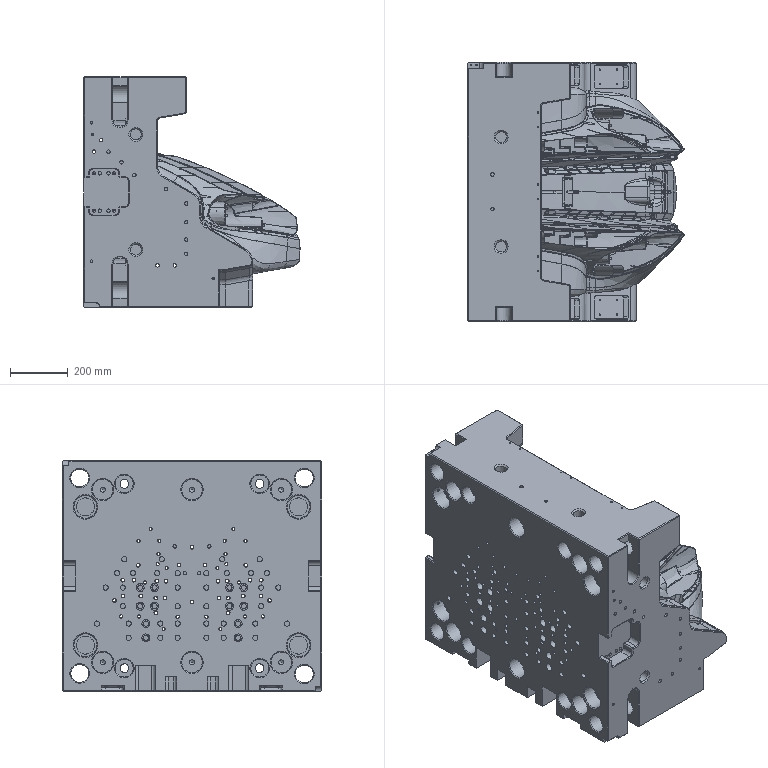Part | STEP file | solid 141 | 1 solid | 4422 faces | volume 250615157 mm3 | spline 1903 | plane 1125 | cylinder 786 | cone 357 | other 107 | sphere 84 | torus 60 | commonest cylinder face diameters 12 x134 16 x96 5 x82 18 x48 13 x36 10 x34